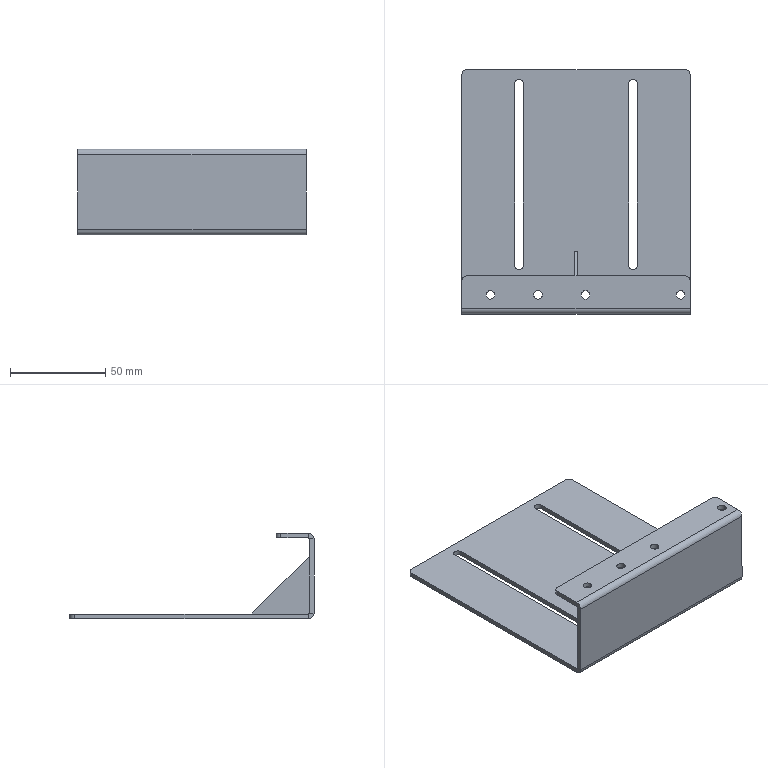Part | SolidWorks | features HoleWzd 3, EdgeFlange 2, Fillet 1, FlatPattern 1, ICE 1, SMBaseFlange 1, SheetMetal 1 | 1 solid | 54 faces | box 120 x 128.5 x 45 mm | volume 54126 mm3 | cylinder 29 | plane 25 | commonest cylinder face diameters 4.5 x12 8 x8 5 x4 1 x3 6 x2